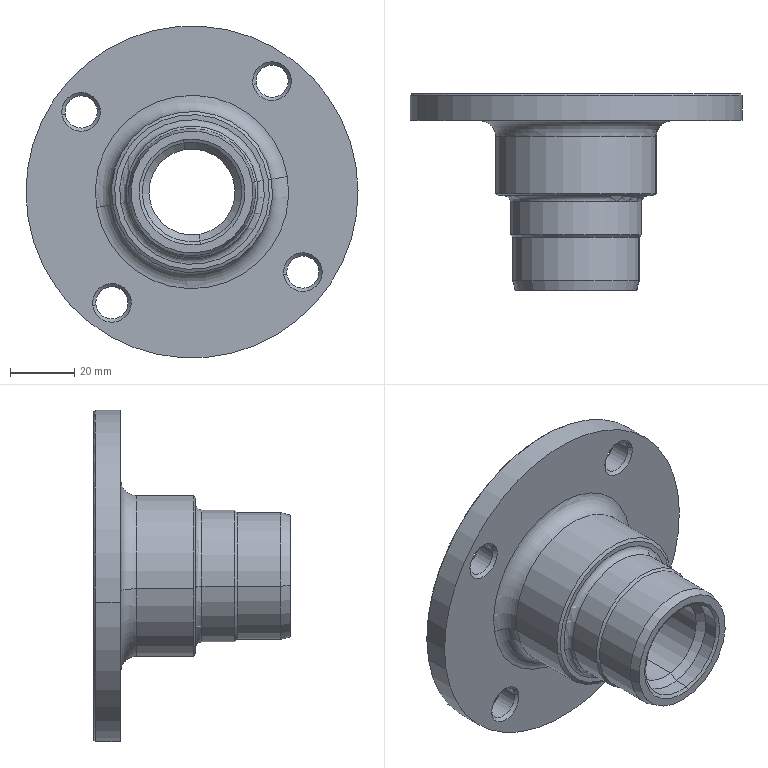Part | NX | features BREP 1 | 1 solid | 68 faces | box 103 x 60.96 x 103 mm | volume 95505 mm3 | cone 32 | cylinder 24 | torus 6 | plane 6 | commonest cylinder face diameters 10 x8 26.703 x2 30.903 x2 39.47 x2 40.403 x2 40.9 x2